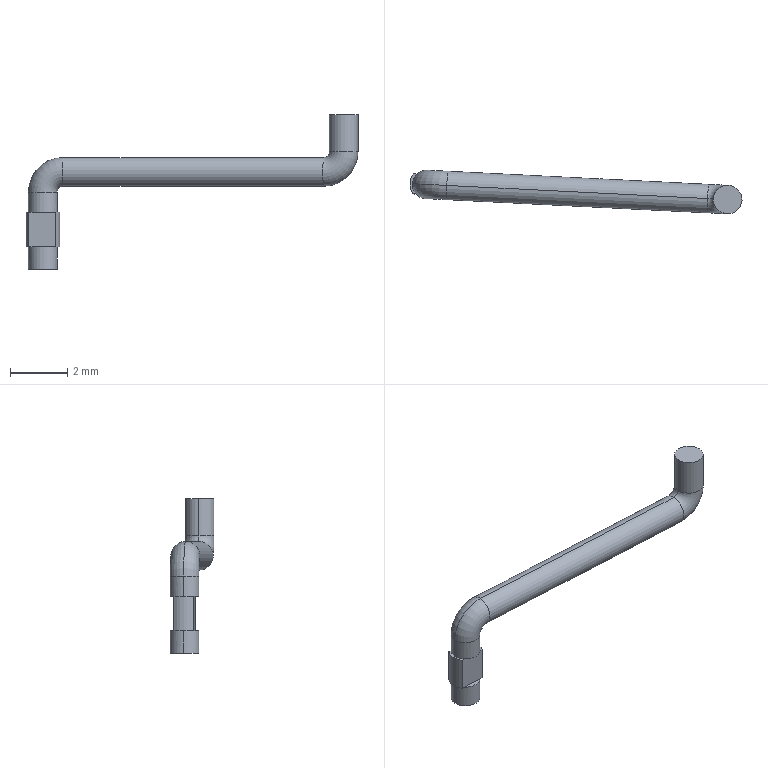Part | NX | features solid 2 | 1 solid | 26 faces | box 11.572 x 1.529 x 5.4 mm | volume 11.994 mm3 | plane 12 | cylinder 10 | torus 4 | commonest cylinder face diameters 1 x8 1.17 x2
STEP:
#1=CARTESIAN_POINT('',(204.831,124.406,-194.01));
#2=VERTEX_POINT('',#1);
#3=CARTESIAN_POINT('',(205.829,124.356,-194.01));
#4=VERTEX_POINT('',#3);
#5=CARTESIAN_POINT('',(205.33,124.381,-194.01));
#6=DIRECTION('',(0.,0.,-1.));
#7=DIRECTION('',(-0.9987,0.05038,0.));
#8=AXIS2_PLACEMENT_3D('',#5,#6,#7);
#9=CIRCLE('',#8,0.5);
#10=EDGE_CURVE('',#2,#4,#9,.T.);
#11=ORIENTED_EDGE('',*,*,#10,.F.);
#12=CARTESIAN_POINT('',(205.33,124.381,-194.01));
#13=DIRECTION('',(0.,0.,-1.));
#14=DIRECTION('',(0.9987,-0.05038,0.));
#15=AXIS2_PLACEMENT_3D('',#12,#13,#14);
#16=CIRCLE('',#15,0.5);
#17=EDGE_CURVE('',#4,#2,#16,.T.);
#18=ORIENTED_EDGE('',*,*,#17,.F.);
#19=EDGE_LOOP('',(#11,#18));
#20=FACE_BOUND('',#19,.T.);
#21=CARTESIAN_POINT('',(205.33,124.381,-194.01));
#22=DIRECTION('',(0.,0.,-1.));
#23=DIRECTION('',(-0.9987,0.05038,0.));
#24=AXIS2_PLACEMENT_3D('',#21,#22,#23);
#25=PLANE('',#24);
#26=ADVANCED_FACE('',(#20),#25,.F.);
#27=CARTESIAN_POINT('',(204.831,124.406,-195.31));
#28=VERTEX_POINT('',#27);
#29=CARTESIAN_POINT('',(204.831,124.406,-195.31));
#30=DIRECTION('',(0.,0.,1.));
#31=VECTOR('',#30,1000.);
#32=LINE('',#29,#31);
#33=EDGE_CURVE('',#28,#2,#32,.T.);
#34=ORIENTED_EDGE('',*,*,#33,.F.);
#35=CARTESIAN_POINT('',(205.829,124.356,-195.31));
#36=VERTEX_POINT('',#35);
#37=CARTESIAN_POINT('',(205.33,124.381,-195.31));
#38=DIRECTION('',(0.,0.,1.));
#39=DIRECTION('',(-0.9987,0.05038,0.));
#40=AXIS2_PLACEMENT_3D('',#37,#38,#39);
#41=CIRCLE('',#40,0.5);
#42=EDGE_CURVE('',#28,#36,#41,.T.);
#43=ORIENTED_EDGE('',*,*,#42,.T.);
#44=CARTESIAN_POINT('',(205.829,124.356,-195.31));
#45=DIRECTION('',(0.,0.,1.));
#46=VECTOR('',#45,1000.);
#47=LINE('',#44,#46);
#48=EDGE_CURVE('',#4,#36,#47,.F.);
#49=ORIENTED_EDGE('',*,*,#48,.F.);
#50=ORIENTED_EDGE('',*,*,#17,.T.);
#51=EDGE_LOOP('',(#34,#43,#49,#50));
#52=FACE_BOUND('',#51,.T.);
#53=CARTESIAN_POINT('',(205.33,124.381,-194.01));
#54=DIRECTION('',(0.,0.,-1.));
#55=DIRECTION('',(-0.9987,0.05038,0.));
#56=AXIS2_PLACEMENT_3D('',#53,#54,#55);
#57=CYLINDRICAL_SURFACE('',#56,0.5);
#58=ADVANCED_FACE('',(#52),#57,.T.);
#59=ORIENTED_EDGE('',*,*,#48,.T.);
#60=CARTESIAN_POINT('',(205.33,124.381,-195.31));
#61=DIRECTION('',(0.,0.,1.));
#62=DIRECTION('',(0.9987,-0.05038,0.));
#63=AXIS2_PLACEMENT_3D('',#60,#61,#62);
#64=CIRCLE('',#63,0.5);
#65=EDGE_CURVE('',#36,#28,#64,.T.);
#66=ORIENTED_EDGE('',*,*,#65,.T.);
#67=ORIENTED_EDGE('',*,*,#33,.T.);
#68=ORIENTED_EDGE('',*,*,#10,.T.);
#69=EDGE_LOOP('',(#59,#66,#67,#68));
#70=FACE_BOUND('',#69,.T.);
#71=CARTESIAN_POINT('',(205.33,124.381,-194.01));
#72=DIRECTION('',(0.,0.,-1.));
#73=DIRECTION('',(-0.9987,0.05038,0.));
#74=AXIS2_PLACEMENT_3D('',#71,#72,#73);
#75=CYLINDRICAL_SURFACE('',#74,0.5);
#76=ADVANCED_FACE('',(#70),#75,.T.);
#77=CARTESIAN_POINT('',(204.631,124.416,-196.51));
#78=VERTEX_POINT('',#77);
#79=CARTESIAN_POINT('',(204.631,124.416,-195.31));
#80=DIRECTION('',(-0.05038,-0.9987,0.));
#81=DIRECTION('',(0.,0.,-1.));
#82=AXIS2_PLACEMENT_3D('',#79,#80,#81);
#83=CIRCLE('',#82,1.2);
#84=EDGE_CURVE('',#36,#78,#83,.F.);
#85=ORIENTED_EDGE('',*,*,#84,.T.);
#86=CARTESIAN_POINT('',(204.631,124.416,-195.51));
#87=VERTEX_POINT('',#86);
#88=CARTESIAN_POINT('',(204.631,124.416,-196.01));
#89=DIRECTION('',(-0.9987,0.05038,0.));
#90=DIRECTION('',(0.,0.,1.));
#91=AXIS2_PLACEMENT_3D('',#88,#89,#90);
#92=CIRCLE('',#91,0.5);
#93=EDGE_CURVE('',#87,#78,#92,.T.);
#94=ORIENTED_EDGE('',*,*,#93,.F.);
#95=CARTESIAN_POINT('',(204.631,124.416,-195.31));
#96=DIRECTION('',(-0.05038,-0.9987,0.));
#97=DIRECTION('',(0.,0.,-1.));
#98=AXIS2_PLACEMENT_3D('',#95,#96,#97);
#99=CIRCLE('',#98,0.2);
#100=EDGE_CURVE('',#87,#28,#99,.T.);
#101=ORIENTED_EDGE('',*,*,#100,.T.);
#102=ORIENTED_EDGE('',*,*,#65,.F.);
#103=EDGE_LOOP('',(#85,#94,#101,#102));
#104=FACE_BOUND('',#103,.T.);
#105=CARTESIAN_POINT('',(204.631,124.416,-195.31));
#106=DIRECTION('',(0.05038,0.9987,0.));
#107=DIRECTION('',(0.9987,-0.05038,0.));
#108=AXIS2_PLACEMENT_3D('',#105,#106,#107);
#109=TOROIDAL_SURFACE('',#108,0.7,0.5);
#110=ADVANCED_FACE('',(#104),#109,.T.);
#111=ORIENTED_EDGE('',*,*,#100,.F.);
#112=CARTESIAN_POINT('',(204.631,124.416,-196.01));
#113=DIRECTION('',(-0.9987,0.05038,0.));
#114=DIRECTION('',(0.,0.,-1.));
#115=AXIS2_PLACEMENT_3D('',#112,#113,#114);
#116=CIRCLE('',#115,0.5);
#117=EDGE_CURVE('',#78,#87,#116,.T.);
#118=ORIENTED_EDGE('',*,*,#117,.F.);
#119=ORIENTED_EDGE('',*,*,#84,.F.);
#120=ORIENTED_EDGE('',*,*,#42,.F.);
#121=EDGE_LOOP('',(#111,#118,#119,#120));
#122=FACE_BOUND('',#121,.T.);
#123=CARTESIAN_POINT('',(204.631,124.416,-195.31));
#124=DIRECTION('',(0.05038,0.9987,0.));
#125=DIRECTION('',(0.9987,-0.05038,0.));
#126=AXIS2_PLACEMENT_3D('',#123,#124,#125);
#127=TOROIDAL_SURFACE('',#126,0.7,0.5);
#128=ADVANCED_FACE('',(#122),#127,.T.);
#129=CARTESIAN_POINT('',(195.542,124.875,-195.51));
#130=VERTEX_POINT('',#129);
#131=CARTESIAN_POINT('',(195.542,124.875,-195.51));
#132=DIRECTION('',(0.9987,-0.05038,0.));
#133=VECTOR('',#132,1000.);
#134=LINE('',#131,#133);
#135=EDGE_CURVE('',#87,#130,#134,.F.);
#136=ORIENTED_EDGE('',*,*,#135,.T.);
#137=CARTESIAN_POINT('',(195.542,124.875,-196.51));
#138=VERTEX_POINT('',#137);
#139=CARTESIAN_POINT('',(195.542,124.875,-196.01));
#140=DIRECTION('',(0.9987,-0.05038,0.));
#141=DIRECTION('',(0.,0.,1.));
#142=AXIS2_PLACEMENT_3D('',#139,#140,#141);
#143=CIRCLE('',#142,0.5);
#144=EDGE_CURVE('',#130,#138,#143,.T.);
#145=ORIENTED_EDGE('',*,*,#144,.T.);
#146=CARTESIAN_POINT('',(195.542,124.875,-196.51));
#147=DIRECTION('',(0.9987,-0.05038,0.));
#148=VECTOR('',#147,1000.);
#149=LINE('',#146,#148);
#150=EDGE_CURVE('',#138,#78,#149,.T.);
#151=ORIENTED_EDGE('',*,*,#150,.T.);
#152=ORIENTED_EDGE('',*,*,#117,.T.);
#153=EDGE_LOOP('',(#136,#145,#151,#152));
#154=FACE_BOUND('',#153,.T.);
#155=CARTESIAN_POINT('',(204.631,124.416,-196.01));
#156=DIRECTION('',(-0.9987,0.05038,0.));
#157=DIRECTION('',(0.,0.,1.));
#158=AXIS2_PLACEMENT_3D('',#155,#156,#157);
#159=CYLINDRICAL_SURFACE('',#158,0.5);
#160=ADVANCED_FACE('',(#154),#159,.T.);
#161=ORIENTED_EDGE('',*,*,#150,.F.);
#162=CARTESIAN_POINT('',(195.542,124.875,-196.01));
#163=DIRECTION('',(0.9987,-0.05038,0.));
#164=DIRECTION('',(0.,0.,-1.));
#165=AXIS2_PLACEMENT_3D('',#162,#163,#164);
#166=CIRCLE('',#165,0.5);
#167=EDGE_CURVE('',#138,#130,#166,.T.);
#168=ORIENTED_EDGE('',*,*,#167,.T.);
#169=ORIENTED_EDGE('',*,*,#135,.F.);
#170=ORIENTED_EDGE('',*,*,#93,.T.);
#171=EDGE_LOOP('',(#161,#168,#169,#170));
#172=FACE_BOUND('',#171,.T.);
#173=CARTESIAN_POINT('',(204.631,124.416,-196.01));
#174=DIRECTION('',(-0.9987,0.05038,0.));
#175=DIRECTION('',(0.,0.,1.));
#176=AXIS2_PLACEMENT_3D('',#173,#174,#175);
#177=CYLINDRICAL_SURFACE('',#176,0.5);
#178=ADVANCED_FACE('',(#172),#177,.T.);
#179=CARTESIAN_POINT('',(195.343,124.885,-196.71));
#180=VERTEX_POINT('',#179);
#181=CARTESIAN_POINT('',(195.542,124.875,-196.71));
#182=DIRECTION('',(0.05038,0.9987,0.));
#183=DIRECTION('',(-0.9987,0.05038,0.));
#184=AXIS2_PLACEMENT_3D('',#181,#182,#183);
#185=CIRCLE('',#184,0.2);
#186=EDGE_CURVE('',#138,#180,#185,.F.);
#187=ORIENTED_EDGE('',*,*,#186,.T.);
#188=CARTESIAN_POINT('',(194.344,124.935,-196.71));
#189=VERTEX_POINT('',#188);
#190=CARTESIAN_POINT('',(194.843,124.91,-196.71));
#191=DIRECTION('',(0.,0.,-1.));
#192=DIRECTION('',(-0.9987,0.05038,0.));
#193=AXIS2_PLACEMENT_3D('',#190,#191,#192);
#194=CIRCLE('',#193,0.5);
#195=EDGE_CURVE('',#189,#180,#194,.T.);
#196=ORIENTED_EDGE('',*,*,#195,.F.);
#197=CARTESIAN_POINT('',(195.542,124.875,-196.71));
#198=DIRECTION('',(0.05038,0.9987,0.));
#199=DIRECTION('',(-0.9987,0.05038,0.));
#200=AXIS2_PLACEMENT_3D('',#197,#198,#199);
#201=CIRCLE('',#200,1.2);
#202=EDGE_CURVE('',#189,#130,#201,.T.);
#203=ORIENTED_EDGE('',*,*,#202,.T.);
#204=ORIENTED_EDGE('',*,*,#167,.F.);
#205=EDGE_LOOP('',(#187,#196,#203,#204));
#206=FACE_BOUND('',#205,.T.);
#207=CARTESIAN_POINT('',(195.542,124.875,-196.71));
#208=DIRECTION('',(-0.05038,-0.9987,0.));
#209=DIRECTION('',(0.,0.,1.));
#210=AXIS2_PLACEMENT_3D('',#207,#208,#209);
#211=TOROIDAL_SURFACE('',#210,0.7,0.5);
#212=ADVANCED_FACE('',(#206),#211,.T.);
#213=ORIENTED_EDGE('',*,*,#202,.F.);
#214=CARTESIAN_POINT('',(194.843,124.91,-196.71));
#215=DIRECTION('',(0.,0.,-1.));
#216=DIRECTION('',(0.9987,-0.05038,0.));
#217=AXIS2_PLACEMENT_3D('',#214,#215,#216);
#218=CIRCLE('',#217,0.5);
#219=EDGE_CURVE('',#180,#189,#218,.T.);
#220=ORIENTED_EDGE('',*,*,#219,.F.);
#221=ORIENTED_EDGE('',*,*,#186,.F.);
#222=ORIENTED_EDGE('',*,*,#144,.F.);
#223=EDGE_LOOP('',(#213,#220,#221,#222));
#224=FACE_BOUND('',#223,.T.);
#225=CARTESIAN_POINT('',(195.542,124.875,-196.71));
#226=DIRECTION('',(-0.05038,-0.9987,0.));
#227=DIRECTION('',(0.,0.,1.));
#228=AXIS2_PLACEMENT_3D('',#225,#226,#227);
#229=TOROIDAL_SURFACE('',#228,0.7,0.5);
#230=ADVANCED_FACE('',(#224),#229,.T.);
#231=CARTESIAN_POINT('',(195.182,124.542,-197.41));
#232=VERTEX_POINT('',#231);
#233=CARTESIAN_POINT('',(195.343,124.885,-197.41));
#234=VERTEX_POINT('',#233);
#235=CARTESIAN_POINT('',(194.843,124.91,-197.41));
#236=DIRECTION('',(0.,0.,1.));
#237=DIRECTION('',(0.678,-0.7351,0.));
#238=AXIS2_PLACEMENT_3D('',#235,#236,#237);
#239=CIRCLE('',#238,0.5);
#240=EDGE_CURVE('',#232,#234,#239,.T.);
#241=ORIENTED_EDGE('',*,*,#240,.T.);
#242=CARTESIAN_POINT('',(195.343,124.885,-197.41));
#243=DIRECTION('',(0.,0.,1.));
#244=VECTOR('',#243,1000.);
#245=LINE('',#242,#244);
#246=EDGE_CURVE('',#180,#234,#245,.F.);
#247=ORIENTED_EDGE('',*,*,#246,.F.);
#248=ORIENTED_EDGE('',*,*,#219,.T.);
#249=CARTESIAN_POINT('',(194.344,124.935,-197.41));
#250=VERTEX_POINT('',#249);
#251=CARTESIAN_POINT('',(194.344,124.935,-197.41));
#252=DIRECTION('',(0.,0.,1.));
#253=VECTOR('',#252,1000.);
#254=LINE('',#251,#253);
#255=EDGE_CURVE('',#250,#189,#254,.T.);
#256=ORIENTED_EDGE('',*,*,#255,.F.);
#257=CARTESIAN_POINT('',(194.469,124.578,-197.41));
#258=VERTEX_POINT('',#257);
#259=CARTESIAN_POINT('',(194.843,124.91,-197.41));
#260=DIRECTION('',(0.,0.,1.));
#261=DIRECTION('',(-0.9987,0.05038,0.));
#262=AXIS2_PLACEMENT_3D('',#259,#260,#261);
#263=CIRCLE('',#262,0.5);
#264=EDGE_CURVE('',#250,#258,#263,.T.);
#265=ORIENTED_EDGE('',*,*,#264,.T.);
#266=CARTESIAN_POINT('',(194.843,124.91,-197.41));
#267=DIRECTION('',(0.,0.,1.));
#268=DIRECTION('',(-0.7485,-0.6631,0.));
#269=AXIS2_PLACEMENT_3D('',#266,#267,#268);
#270=CIRCLE('',#269,0.5);
#271=EDGE_CURVE('',#258,#232,#270,.T.);
#272=ORIENTED_EDGE('',*,*,#271,.T.);
#273=EDGE_LOOP('',(#241,#247,#248,#256,#265,#272));
#274=FACE_BOUND('',#273,.T.);
#275=CARTESIAN_POINT('',(194.843,124.91,-196.71));
#276=DIRECTION('',(0.,0.,-1.));
#277=DIRECTION('',(-0.9987,0.05038,0.));
#278=AXIS2_PLACEMENT_3D('',#275,#276,#277);
#279=CYLINDRICAL_SURFACE('',#278,0.5);
#280=ADVANCED_FACE('',(#274),#279,.T.);
#281=CARTESIAN_POINT('',(195.182,124.542,-197.41));
#282=DIRECTION('',(-0.9987,0.05038,0.));
#283=VECTOR('',#282,1000.);
#284=LINE('',#281,#283);
#285=EDGE_CURVE('',#232,#258,#284,.T.);
#286=ORIENTED_EDGE('',*,*,#285,.F.);
#287=ORIENTED_EDGE('',*,*,#271,.F.);
#288=EDGE_LOOP('',(#286,#287));
#289=FACE_BOUND('',#288,.T.);
#290=CARTESIAN_POINT('',(194.843,124.91,-197.41));
#291=DIRECTION('',(0.,0.,-1.));
#292=DIRECTION('',(-0.9987,0.05038,0.));
#293=AXIS2_PLACEMENT_3D('',#290,#291,#292);
#294=PLANE('',#293);
#295=ADVANCED_FACE('',(#289),#294,.T.);
#296=CARTESIAN_POINT('',(195.294,124.537,-198.61));
#297=VERTEX_POINT('',#296);
#298=CARTESIAN_POINT('',(195.294,124.537,-197.41));
#299=VERTEX_POINT('',#298);
#300=CARTESIAN_POINT('',(195.294,124.537,-198.61));
#301=DIRECTION('',(0.,0.,1.));
#302=VECTOR('',#301,1000.);
#303=LINE('',#300,#302);
#304=EDGE_CURVE('',#297,#299,#303,.T.);
#305=ORIENTED_EDGE('',*,*,#304,.T.);
#306=CARTESIAN_POINT('',(195.182,124.542,-197.41));
#307=DIRECTION('',(0.9987,-0.05038,0.));
#308=VECTOR('',#307,1000.);
#309=LINE('',#306,#308);
#310=EDGE_CURVE('',#232,#299,#309,.T.);
#311=ORIENTED_EDGE('',*,*,#310,.F.);
#312=ORIENTED_EDGE('',*,*,#285,.T.);
#313=CARTESIAN_POINT('',(194.358,124.584,-197.41));
#314=VERTEX_POINT('',#313);
#315=CARTESIAN_POINT('',(194.358,124.584,-197.41));
#316=DIRECTION('',(0.9987,-0.05038,0.));
#317=VECTOR('',#316,1000.);
#318=LINE('',#315,#317);
#319=EDGE_CURVE('',#314,#258,#318,.T.);
#320=ORIENTED_EDGE('',*,*,#319,.F.);
#321=CARTESIAN_POINT('',(194.358,124.584,-198.61));
#322=VERTEX_POINT('',#321);
#323=CARTESIAN_POINT('',(194.358,124.584,-197.41));
#324=DIRECTION('',(0.,0.,-1.));
#325=VECTOR('',#324,1000.);
#326=LINE('',#323,#325);
#327=EDGE_CURVE('',#314,#322,#326,.T.);
#328=ORIENTED_EDGE('',*,*,#327,.T.);
#329=CARTESIAN_POINT('',(194.469,124.578,-198.61));
#330=VERTEX_POINT('',#329);
#331=CARTESIAN_POINT('',(194.358,124.584,-198.61));
#332=DIRECTION('',(0.9987,-0.05038,0.));
#333=VECTOR('',#332,1000.);
#334=LINE('',#331,#333);
#335=EDGE_CURVE('',#322,#330,#334,.T.);
#336=ORIENTED_EDGE('',*,*,#335,.T.);
#337=CARTESIAN_POINT('',(195.182,124.542,-198.61));
#338=VERTEX_POINT('',#337);
#339=CARTESIAN_POINT('',(195.182,124.542,-198.61));
#340=DIRECTION('',(-0.9987,0.05038,0.));
#341=VECTOR('',#340,1000.);
#342=LINE('',#339,#341);
#343=EDGE_CURVE('',#338,#330,#342,.T.);
#344=ORIENTED_EDGE('',*,*,#343,.F.);
#345=CARTESIAN_POINT('',(195.182,124.542,-198.61));
#346=DIRECTION('',(0.9987,-0.05038,0.));
#347=VECTOR('',#346,1000.);
#348=LINE('',#345,#347);
#349=EDGE_CURVE('',#338,#297,#348,.T.);
#350=ORIENTED_EDGE('',*,*,#349,.T.);
#351=EDGE_LOOP('',(#305,#311,#312,#320,#328,#336,#344,#350));
#352=FACE_BOUND('',#351,.T.);
#353=CARTESIAN_POINT('',(195.294,124.537,-198.61));
#354=DIRECTION('',(-0.05038,-0.9987,0.));
#355=DIRECTION('',(0.9987,-0.05038,0.));
#356=AXIS2_PLACEMENT_3D('',#353,#354,#355);
#357=PLANE('',#356);
#358=ADVANCED_FACE('',(#352),#357,.T.);
#359=CARTESIAN_POINT('',(195.218,125.242,-198.61));
#360=VERTEX_POINT('',#359);
#361=CARTESIAN_POINT('',(195.343,124.885,-198.61));
#362=VERTEX_POINT('',#361);
#363=CARTESIAN_POINT('',(194.843,124.91,-198.61));
#364=DIRECTION('',(0.,0.,-1.));
#365=DIRECTION('',(0.7485,0.6631,0.));
#366=AXIS2_PLACEMENT_3D('',#363,#364,#365);
#367=CIRCLE('',#366,0.5);
#368=EDGE_CURVE('',#360,#362,#367,.T.);
#369=ORIENTED_EDGE('',*,*,#368,.F.);
#370=CARTESIAN_POINT('',(195.329,125.236,-198.61));
#371=VERTEX_POINT('',#370);
#372=CARTESIAN_POINT('',(195.329,125.236,-198.61));
#373=DIRECTION('',(-0.9987,0.05038,0.));
#374=VECTOR('',#373,1000.);
#375=LINE('',#372,#374);
#376=EDGE_CURVE('',#371,#360,#375,.T.);
#377=ORIENTED_EDGE('',*,*,#376,.F.);
#378=CARTESIAN_POINT('',(195.428,124.881,-198.61));
#379=VERTEX_POINT('',#378);
#380=CARTESIAN_POINT('',(194.843,124.91,-198.61));
#381=DIRECTION('',(0.,0.,1.));
#382=DIRECTION('',(0.9987,-0.05038,0.));
#383=AXIS2_PLACEMENT_3D('',#380,#381,#382);
#384=CIRCLE('',#383,0.585);
#385=EDGE_CURVE('',#379,#371,#384,.T.);
#386=ORIENTED_EDGE('',*,*,#385,.F.);
#387=CARTESIAN_POINT('',(194.843,124.91,-198.61));
#388=DIRECTION('',(0.,0.,1.));
#389=DIRECTION('',(0.7701,-0.6379,0.));
#390=AXIS2_PLACEMENT_3D('',#387,#388,#389);
#391=CIRCLE('',#390,0.585);
#392=EDGE_CURVE('',#297,#379,#391,.T.);
#393=ORIENTED_EDGE('',*,*,#392,.F.);
#394=ORIENTED_EDGE('',*,*,#349,.F.);
#395=CARTESIAN_POINT('',(194.843,124.91,-198.61));
#396=DIRECTION('',(0.,0.,-1.));
#397=DIRECTION('',(0.9987,-0.05038,0.));
#398=AXIS2_PLACEMENT_3D('',#395,#396,#397);
#399=CIRCLE('',#398,0.5);
#400=EDGE_CURVE('',#362,#338,#399,.T.);
#401=ORIENTED_EDGE('',*,*,#400,.F.);
#402=EDGE_LOOP('',(#369,#377,#386,#393,#394,#401));
#403=FACE_BOUND('',#402,.T.);
#404=CARTESIAN_POINT('',(194.843,124.91,-198.61));
#405=DIRECTION('',(0.,0.,-1.));
#406=DIRECTION('',(-0.9987,0.05038,0.));
#407=AXIS2_PLACEMENT_3D('',#404,#405,#406);
#408=PLANE('',#407);
#409=ADVANCED_FACE('',(#403),#408,.T.);
#410=CARTESIAN_POINT('',(194.344,124.935,-198.61));
#411=VERTEX_POINT('',#410);
#412=CARTESIAN_POINT('',(194.843,124.91,-198.61));
#413=DIRECTION('',(0.,0.,-1.));
#414=DIRECTION('',(-0.7485,-0.6631,0.));
#415=AXIS2_PLACEMENT_3D('',#412,#413,#414);
#416=CIRCLE('',#415,0.5);
#417=EDGE_CURVE('',#330,#411,#416,.T.);
#418=ORIENTED_EDGE('',*,*,#417,.T.);
#419=CARTESIAN_POINT('',(194.344,124.935,-199.41));
#420=VERTEX_POINT('',#419);
#421=CARTESIAN_POINT('',(194.344,124.935,-199.41));
#422=DIRECTION('',(0.,0.,1.));
#423=VECTOR('',#422,1000.);
#424=LINE('',#421,#423);
#425=EDGE_CURVE('',#411,#420,#424,.F.);
#426=ORIENTED_EDGE('',*,*,#425,.T.);
#427=CARTESIAN_POINT('',(195.343,124.885,-199.41));
#428=VERTEX_POINT('',#427);
#429=CARTESIAN_POINT('',(194.843,124.91,-199.41));
#430=DIRECTION('',(0.,0.,1.));
#431=DIRECTION('',(-0.9987,0.05038,0.));
#432=AXIS2_PLACEMENT_3D('',#429,#430,#431);
#433=CIRCLE('',#432,0.5);
#434=EDGE_CURVE('',#420,#428,#433,.T.);
#435=ORIENTED_EDGE('',*,*,#434,.T.);
#436=CARTESIAN_POINT('',(195.343,124.885,-199.41));
#437=DIRECTION('',(0.,0.,1.));
#438=VECTOR('',#437,1000.);
#439=LINE('',#436,#438);
#440=EDGE_CURVE('',#428,#362,#439,.T.);
#441=ORIENTED_EDGE('',*,*,#440,.T.);
#442=ORIENTED_EDGE('',*,*,#400,.T.);
#443=CARTESIAN_POINT('',(194.843,124.91,-198.61));
#444=DIRECTION('',(0.,0.,-1.));
#445=DIRECTION('',(0.678,-0.7351,0.));
#446=AXIS2_PLACEMENT_3D('',#443,#444,#445);
#447=CIRCLE('',#446,0.5);
#448=EDGE_CURVE('',#338,#330,#447,.T.);
#449=ORIENTED_EDGE('',*,*,#448,.T.);
#450=EDGE_LOOP('',(#418,#426,#435,#441,#442,#449));
#451=FACE_BOUND('',#450,.T.);
#452=CARTESIAN_POINT('',(194.843,124.91,-196.71));
#453=DIRECTION('',(0.,0.,-1.));
#454=DIRECTION('',(-0.9987,0.05038,0.));
#455=AXIS2_PLACEMENT_3D('',#452,#453,#454);
#456=CYLINDRICAL_SURFACE('',#455,0.5);
#457=ADVANCED_FACE('',(#451),#456,.T.);
#458=ORIENTED_EDGE('',*,*,#343,.T.);
#459=ORIENTED_EDGE('',*,*,#448,.F.);
#460=EDGE_LOOP('',(#458,#459));
#461=FACE_BOUND('',#460,.T.);
#462=CARTESIAN_POINT('',(194.843,124.91,-198.61));
#463=DIRECTION('',(0.,0.,-1.));
#464=DIRECTION('',(-0.9987,0.05038,0.));
#465=AXIS2_PLACEMENT_3D('',#462,#463,#464);
#466=PLANE('',#465);
#467=ADVANCED_FACE('',(#461),#466,.F.);
#468=ORIENTED_EDGE('',*,*,#368,.T.);
#469=ORIENTED_EDGE('',*,*,#440,.F.);
#470=CARTESIAN_POINT('',(194.843,124.91,-199.41));
#471=DIRECTION('',(0.,0.,1.));
#472=DIRECTION('',(0.9987,-0.05038,0.));
#473=AXIS2_PLACEMENT_3D('',#470,#471,#472);
#474=CIRCLE('',#473,0.5);
#475=EDGE_CURVE('',#428,#420,#474,.T.);
#476=ORIENTED_EDGE('',*,*,#475,.T.);
#477=ORIENTED_EDGE('',*,*,#425,.F.);
#478=CARTESIAN_POINT('',(194.504,125.278,-198.61));
#479=VERTEX_POINT('',#478);
#480=CARTESIAN_POINT('',(194.843,124.91,-198.61));
#481=DIRECTION('',(0.,0.,-1.));
#482=DIRECTION('',(-0.9987,0.05038,0.));
#483=AXIS2_PLACEMENT_3D('',#480,#481,#482);
#484=CIRCLE('',#483,0.5);
#485=EDGE_CURVE('',#411,#479,#484,.T.);
#486=ORIENTED_EDGE('',*,*,#485,.T.);
#487=CARTESIAN_POINT('',(194.843,124.91,-198.61));
#488=DIRECTION('',(0.,0.,-1.));
#489=DIRECTION('',(-0.678,0.7351,0.));
#490=AXIS2_PLACEMENT_3D('',#487,#488,#489);
#491=CIRCLE('',#490,0.5);
#492=EDGE_CURVE('',#479,#360,#491,.T.);
#493=ORIENTED_EDGE('',*,*,#492,.T.);
#494=EDGE_LOOP('',(#468,#469,#476,#477,#486,#493));
#495=FACE_BOUND('',#494,.T.);
#496=CARTESIAN_POINT('',(194.843,124.91,-196.71));
#497=DIRECTION('',(0.,0.,-1.));
#498=DIRECTION('',(-0.9987,0.05038,0.));
#499=AXIS2_PLACEMENT_3D('',#496,#497,#498);
#500=CYLINDRICAL_SURFACE('',#499,0.5);
#501=ADVANCED_FACE('',(#495),#500,.T.);
#502=CARTESIAN_POINT('',(194.504,125.278,-198.61));
#503=DIRECTION('',(0.9987,-0.05038,0.));
#504=VECTOR('',#503,1000.);
#505=LINE('',#502,#504);
#506=EDGE_CURVE('',#479,#360,#505,.T.);
#507=ORIENTED_EDGE('',*,*,#506,.T.);
#508=ORIENTED_EDGE('',*,*,#492,.F.);
#509=EDGE_LOOP('',(#507,#508));
#510=FACE_BOUND('',#509,.T.);
#511=CARTESIAN_POINT('',(194.843,124.91,-198.61));
#512=DIRECTION('',(0.,0.,-1.));
#513=DIRECTION('',(-0.9987,0.05038,0.));
#514=AXIS2_PLACEMENT_3D('',#511,#512,#513);
#515=PLANE('',#514);
#516=ADVANCED_FACE('',(#510),#515,.F.);
#517=CARTESIAN_POINT('',(194.393,125.283,-198.61));
#518=VERTEX_POINT('',#517);
#519=CARTESIAN_POINT('',(194.393,125.283,-197.41));
#520=VERTEX_POINT('',#519);
#521=CARTESIAN_POINT('',(194.393,125.283,-198.61));
#522=DIRECTION('',(0.,0.,1.));
#523=VECTOR('',#522,1000.);
#524=LINE('',#521,#523);
#525=EDGE_CURVE('',#518,#520,#524,.T.);
#526=ORIENTED_EDGE('',*,*,#525,.T.);
#527=CARTESIAN_POINT('',(194.504,125.278,-197.41));
#528=VERTEX_POINT('',#527);
#529=CARTESIAN_POINT('',(194.504,125.278,-197.41));
#530=DIRECTION('',(-0.9987,0.05038,0.));
#531=VECTOR('',#530,1000.);
#532=LINE('',#529,#531);
#533=EDGE_CURVE('',#528,#520,#532,.T.);
#534=ORIENTED_EDGE('',*,*,#533,.F.);
#535=CARTESIAN_POINT('',(195.218,125.242,-197.41));
#536=VERTEX_POINT('',#535);
#537=CARTESIAN_POINT('',(194.504,125.278,-197.41));
#538=DIRECTION('',(0.9987,-0.05038,0.));
#539=VECTOR('',#538,1000.);
#540=LINE('',#537,#539);
#541=EDGE_CURVE('',#528,#536,#540,.T.);
#542=ORIENTED_EDGE('',*,*,#541,.T.);
#543=CARTESIAN_POINT('',(195.329,125.236,-197.41));
#544=VERTEX_POINT('',#543);
#545=CARTESIAN_POINT('',(195.329,125.236,-197.41));
#546=DIRECTION('',(-0.9987,0.05038,0.));
#547=VECTOR('',#546,1000.);
#548=LINE('',#545,#547);
#549=EDGE_CURVE('',#544,#536,#548,.T.);
#550=ORIENTED_EDGE('',*,*,#549,.F.);
#551=CARTESIAN_POINT('',(195.329,125.236,-197.41));
#552=DIRECTION('',(0.,0.,-1.));
#553=VECTOR('',#552,1000.);
#554=LINE('',#551,#553);
#555=EDGE_CURVE('',#544,#371,#554,.T.);
#556=ORIENTED_EDGE('',*,*,#555,.T.);
#557=ORIENTED_EDGE('',*,*,#376,.T.);
#558=ORIENTED_EDGE('',*,*,#506,.F.);
#559=CARTESIAN_POINT('',(194.504,125.278,-198.61));
#560=DIRECTION('',(-0.9987,0.05038,0.));
#561=VECTOR('',#560,1000.);
#562=LINE('',#559,#561);
#563=EDGE_CURVE('',#479,#518,#562,.T.);
#564=ORIENTED_EDGE('',*,*,#563,.T.);
#565=EDGE_LOOP('',(#526,#534,#542,#550,#556,#557,#558,#564));
#566=FACE_BOUND('',#565,.T.);
#567=CARTESIAN_POINT('',(194.393,125.283,-198.61));
#568=DIRECTION('',(0.05038,0.9987,0.));
#569=DIRECTION('',(-0.9987,0.05038,0.));
#570=AXIS2_PLACEMENT_3D('',#567,#568,#569);
#571=PLANE('',#570);
#572=ADVANCED_FACE('',(#566),#571,.T.);
#573=ORIENTED_EDGE('',*,*,#335,.F.);
#574=CARTESIAN_POINT('',(194.259,124.939,-198.61));
#575=VERTEX_POINT('',#574);
#576=CARTESIAN_POINT('',(194.843,124.91,-198.61));
#577=DIRECTION('',(0.,0.,1.));
#578=DIRECTION('',(-0.9987,0.05038,0.));
#579=AXIS2_PLACEMENT_3D('',#576,#577,#578);
#580=CIRCLE('',#579,0.585);
#581=EDGE_CURVE('',#575,#322,#580,.T.);
#582=ORIENTED_EDGE('',*,*,#581,.F.);
#583=CARTESIAN_POINT('',(194.843,124.91,-198.61));
#584=DIRECTION('',(0.,0.,1.));
#585=DIRECTION('',(-0.7701,0.6379,0.));
#586=AXIS2_PLACEMENT_3D('',#583,#584,#585);
#587=CIRCLE('',#586,0.585);
#588=EDGE_CURVE('',#518,#575,#587,.T.);
#589=ORIENTED_EDGE('',*,*,#588,.F.);
#590=ORIENTED_EDGE('',*,*,#563,.F.);
#591=ORIENTED_EDGE('',*,*,#485,.F.);
#592=ORIENTED_EDGE('',*,*,#417,.F.);
#593=EDGE_LOOP('',(#573,#582,#589,#590,#591,#592));
#594=FACE_BOUND('',#593,.T.);
#595=CARTESIAN_POINT('',(194.843,124.91,-198.61));
#596=DIRECTION('',(0.,0.,-1.));
#597=DIRECTION('',(-0.9987,0.05038,0.));
#598=AXIS2_PLACEMENT_3D('',#595,#596,#597);
#599=PLANE('',#598);
#600=ADVANCED_FACE('',(#594),#599,.T.);
#601=ORIENTED_EDGE('',*,*,#327,.F.);
#602=CARTESIAN_POINT('',(194.259,124.939,-197.41));
#603=VERTEX_POINT('',#602);
#604=CARTESIAN_POINT('',(194.843,124.91,-197.41));
#605=DIRECTION('',(0.,0.,-1.));
#606=DIRECTION('',(-0.8304,-0.5572,0.));
#607=AXIS2_PLACEMENT_3D('',#604,#605,#606);
#608=CIRCLE('',#607,0.585);
#609=EDGE_CURVE('',#314,#603,#608,.T.);
#610=ORIENTED_EDGE('',*,*,#609,.T.);
#611=CARTESIAN_POINT('',(194.843,124.91,-197.41));
#612=DIRECTION('',(0.,0.,-1.));
#613=DIRECTION('',(-0.9987,0.05038,0.));
#614=AXIS2_PLACEMENT_3D('',#611,#612,#613);
#615=CIRCLE('',#614,0.585);
#616=EDGE_CURVE('',#603,#520,#615,.T.);
#617=ORIENTED_EDGE('',*,*,#616,.T.);
#618=ORIENTED_EDGE('',*,*,#525,.F.);
#619=ORIENTED_EDGE('',*,*,#588,.T.);
#620=ORIENTED_EDGE('',*,*,#581,.T.);
#621=EDGE_LOOP('',(#601,#610,#617,#618,#619,#620));
#622=FACE_BOUND('',#621,.T.);
#623=CARTESIAN_POINT('',(194.843,124.91,-198.61));
#624=DIRECTION('',(0.,0.,-1.));
#625=DIRECTION('',(-0.9987,0.05038,0.));
#626=AXIS2_PLACEMENT_3D('',#623,#624,#625);
#627=CYLINDRICAL_SURFACE('',#626,0.585);
#628=ADVANCED_FACE('',(#622),#627,.T.);
#629=CARTESIAN_POINT('',(194.843,124.91,-197.41));
#630=DIRECTION('',(0.,0.,1.));
#631=DIRECTION('',(-0.678,0.7351,0.));
#632=AXIS2_PLACEMENT_3D('',#629,#630,#631);
#633=CIRCLE('',#632,0.5);
#634=EDGE_CURVE('',#528,#250,#633,.T.);
#635=ORIENTED_EDGE('',*,*,#634,.F.);
#636=ORIENTED_EDGE('',*,*,#533,.T.);
#637=ORIENTED_EDGE('',*,*,#616,.F.);
#638=ORIENTED_EDGE('',*,*,#609,.F.);
#639=ORIENTED_EDGE('',*,*,#319,.T.);
#640=ORIENTED_EDGE('',*,*,#264,.F.);
#641=EDGE_LOOP('',(#635,#636,#637,#638,#639,#640));
#642=FACE_BOUND('',#641,.T.);
#643=CARTESIAN_POINT('',(194.843,124.91,-197.41));
#644=DIRECTION('',(0.,0.,-1.));
#645=DIRECTION('',(-0.9987,0.05038,0.));
#646=AXIS2_PLACEMENT_3D('',#643,#644,#645);
#647=PLANE('',#646);
#648=ADVANCED_FACE('',(#642),#647,.F.);
#649=ORIENTED_EDGE('',*,*,#634,.T.);
#650=ORIENTED_EDGE('',*,*,#255,.T.);
#651=ORIENTED_EDGE('',*,*,#195,.T.);
#652=ORIENTED_EDGE('',*,*,#246,.T.);
#653=CARTESIAN_POINT('',(194.843,124.91,-197.41));
#654=DIRECTION('',(0.,0.,1.));
#655=DIRECTION('',(0.9987,-0.05038,0.));
#656=AXIS2_PLACEMENT_3D('',#653,#654,#655);
#657=CIRCLE('',#656,0.5);
#658=EDGE_CURVE('',#234,#536,#657,.T.);
#659=ORIENTED_EDGE('',*,*,#658,.T.);
#660=CARTESIAN_POINT('',(194.843,124.91,-197.41));
#661=DIRECTION('',(0.,0.,1.));
#662=DIRECTION('',(0.7485,0.6631,0.));
#663=AXIS2_PLACEMENT_3D('',#660,#661,#662);
#664=CIRCLE('',#663,0.5);
#665=EDGE_CURVE('',#536,#528,#664,.T.);
#666=ORIENTED_EDGE('',*,*,#665,.T.);
#667=EDGE_LOOP('',(#649,#650,#651,#652,#659,#666));
#668=FACE_BOUND('',#667,.T.);
#669=CARTESIAN_POINT('',(194.843,124.91,-196.71));
#670=DIRECTION('',(0.,0.,-1.));
#671=DIRECTION('',(-0.9987,0.05038,0.));
#672=AXIS2_PLACEMENT_3D('',#669,#670,#671);
#673=CYLINDRICAL_SURFACE('',#672,0.5);
#674=ADVANCED_FACE('',(#668),#673,.T.);
#675=ORIENTED_EDGE('',*,*,#541,.F.);
#676=ORIENTED_EDGE('',*,*,#665,.F.);
#677=EDGE_LOOP('',(#675,#676));
#678=FACE_BOUND('',#677,.T.);
#679=CARTESIAN_POINT('',(194.843,124.91,-197.41));
#680=DIRECTION('',(0.,0.,-1.));
#681=DIRECTION('',(-0.9987,0.05038,0.));
#682=AXIS2_PLACEMENT_3D('',#679,#680,#681);
#683=PLANE('',#682);
#684=ADVANCED_FACE('',(#678),#683,.T.);
#685=ORIENTED_EDGE('',*,*,#310,.T.);
#686=CARTESIAN_POINT('',(195.428,124.881,-197.41));
#687=VERTEX_POINT('',#686);
#688=CARTESIAN_POINT('',(194.843,124.91,-197.41));
#689=DIRECTION('',(0.,0.,-1.));
#690=DIRECTION('',(0.9987,-0.05038,0.));
#691=AXIS2_PLACEMENT_3D('',#688,#689,#690);
#692=CIRCLE('',#691,0.585);
#693=EDGE_CURVE('',#687,#299,#692,.T.);
#694=ORIENTED_EDGE('',*,*,#693,.F.);
#695=CARTESIAN_POINT('',(194.843,124.91,-197.41));
#696=DIRECTION('',(0.,0.,-1.));
#697=DIRECTION('',(0.8304,0.5572,0.));
#698=AXIS2_PLACEMENT_3D('',#695,#696,#697);
#699=CIRCLE('',#698,0.585);
#700=EDGE_CURVE('',#544,#687,#699,.T.);
#701=ORIENTED_EDGE('',*,*,#700,.F.);
#702=ORIENTED_EDGE('',*,*,#549,.T.);
#703=ORIENTED_EDGE('',*,*,#658,.F.);
#704=ORIENTED_EDGE('',*,*,#240,.F.);
#705=EDGE_LOOP('',(#685,#694,#701,#702,#703,#704));
#706=FACE_BOUND('',#705,.T.);
#707=CARTESIAN_POINT('',(194.843,124.91,-197.41));
#708=DIRECTION('',(0.,0.,-1.));
#709=DIRECTION('',(-0.9987,0.05038,0.));
#710=AXIS2_PLACEMENT_3D('',#707,#708,#709);
#711=PLANE('',#710);
#712=ADVANCED_FACE('',(#706),#711,.F.);
#713=ORIENTED_EDGE('',*,*,#555,.F.);
#714=ORIENTED_EDGE('',*,*,#700,.T.);
#715=ORIENTED_EDGE('',*,*,#693,.T.);
#716=ORIENTED_EDGE('',*,*,#304,.F.);
#717=ORIENTED_EDGE('',*,*,#392,.T.);
#718=ORIENTED_EDGE('',*,*,#385,.T.);
#719=EDGE_LOOP('',(#713,#714,#715,#716,#717,#718));
#720=FACE_BOUND('',#719,.T.);
#721=CARTESIAN_POINT('',(194.843,124.91,-198.61));
#722=DIRECTION('',(0.,0.,-1.));
#723=DIRECTION('',(-0.9987,0.05038,0.));
#724=AXIS2_PLACEMENT_3D('',#721,#722,#723);
#725=CYLINDRICAL_SURFACE('',#724,0.585);
#726=ADVANCED_FACE('',(#720),#725,.T.);
#727=ORIENTED_EDGE('',*,*,#475,.F.);
#728=ORIENTED_EDGE('',*,*,#434,.F.);
#729=EDGE_LOOP('',(#727,#728));
#730=FACE_BOUND('',#729,.T.);
#731=CARTESIAN_POINT('',(194.843,124.91,-199.41));
#732=DIRECTION('',(0.,0.,-1.));
#733=DIRECTION('',(-0.9987,0.05038,0.));
#734=AXIS2_PLACEMENT_3D('',#731,#732,#733);
#735=PLANE('',#734);
#736=ADVANCED_FACE('',(#730),#735,.T.);
#737=CLOSED_SHELL('',(#26,#58,#76,#110,#128,#160,#178,#212,#230,#280,#295,#358,#409,#457,#467,#501,#516,#572,#600,#628,#648,#674,#684,#712,#726,#736));
#738=MANIFOLD_SOLID_BREP('',#737);
#739=(LENGTH_UNIT()NAMED_UNIT(*)SI_UNIT(.MILLI.,.METRE.));
#740=UNCERTAINTY_MEASURE_WITH_UNIT(LENGTH_MEASURE(0.00001),#739,'','');
#741=(NAMED_UNIT(*)PLANE_ANGLE_UNIT()SI_UNIT($,.RADIAN.));
#742=(NAMED_UNIT(*)SI_UNIT($,.STERADIAN.)SOLID_ANGLE_UNIT());
#743=(GEOMETRIC_REPRESENTATION_CONTEXT(3)GLOBAL_UNCERTAINTY_ASSIGNED_CONTEXT((#740))GLOBAL_UNIT_ASSIGNED_CONTEXT((#739,#741,#742))REPRESENTATION_CONTEXT('',''));
#744=ADVANCED_BREP_SHAPE_REPRESENTATION('',(#738),#743);